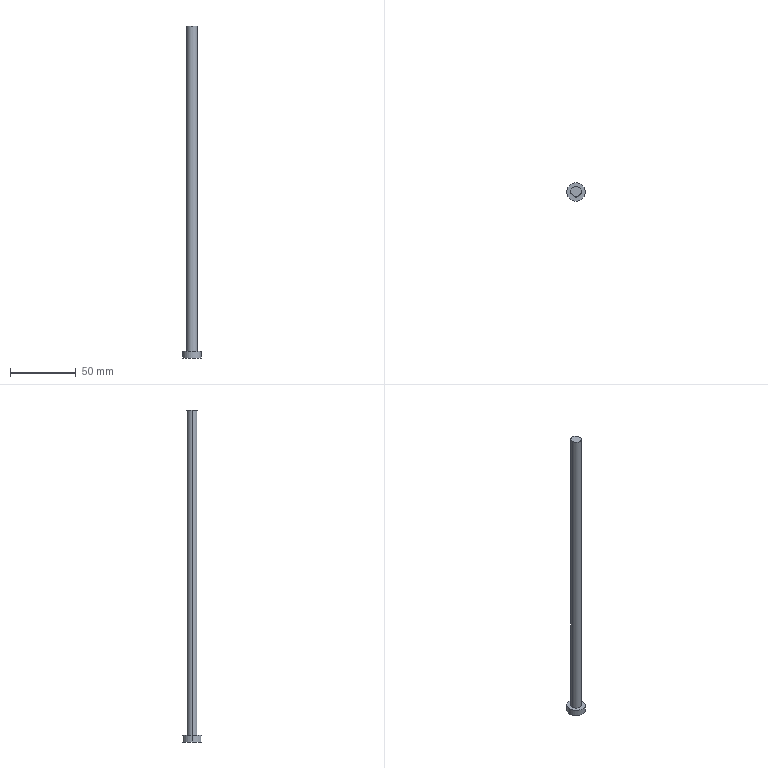Part | Creo | 1 solid | 7 faces | box 14 x 14 x 252.352 mm | volume 13203 mm3 | cylinder 4 | plane 3 | commonest cylinder face diameters 8 x2 14 x2
STEP:
#1=CARTESIAN_POINT('',(4.,0.,26.852));
#2=VERTEX_POINT('',#1);
#3=CARTESIAN_POINT('',(-4.,0.,26.852));
#4=VERTEX_POINT('',#3);
#5=CARTESIAN_POINT('',(0.,0.,26.852));
#6=DIRECTION('',(0.,0.,1.));
#7=DIRECTION('',(1.,0.,0.));
#8=AXIS2_PLACEMENT_3D('',#5,#6,#7);
#9=CIRCLE('',#8,4.);
#10=EDGE_CURVE('',#2,#4,#9,.T.);
#11=ORIENTED_EDGE('',*,*,#10,.T.);
#12=CARTESIAN_POINT('',(-4.,0.,-220.5));
#13=VERTEX_POINT('',#12);
#14=CARTESIAN_POINT('',(-4.,0.,26.852));
#15=DIRECTION('',(0.,0.,-1.));
#16=VECTOR('',#15,247.352);
#17=LINE('',#14,#16);
#18=EDGE_CURVE('',#4,#13,#17,.T.);
#19=ORIENTED_EDGE('',*,*,#18,.T.);
#20=CARTESIAN_POINT('',(4.,0.,-220.5));
#21=VERTEX_POINT('',#20);
#22=CARTESIAN_POINT('',(0.,0.,-220.5));
#23=DIRECTION('',(0.,0.,-1.));
#24=DIRECTION('',(-1.,0.,0.));
#25=AXIS2_PLACEMENT_3D('',#22,#23,#24);
#26=CIRCLE('',#25,4.);
#27=EDGE_CURVE('',#13,#21,#26,.T.);
#28=ORIENTED_EDGE('',*,*,#27,.T.);
#29=CARTESIAN_POINT('',(4.,0.,26.852));
#30=DIRECTION('',(0.,0.,-1.));
#31=VECTOR('',#30,247.352);
#32=LINE('',#29,#31);
#33=EDGE_CURVE('',#2,#21,#32,.T.);
#34=ORIENTED_EDGE('',*,*,#33,.F.);
#35=EDGE_LOOP('',(#11,#19,#28,#34));
#36=FACE_OUTER_BOUND('',#35,.F.);
#37=CARTESIAN_POINT('',(0.,0.,49.5));
#38=DIRECTION('',(0.,0.,-1.));
#39=DIRECTION('',(-1.,0.,0.));
#40=AXIS2_PLACEMENT_3D('',#37,#38,#39);
#41=CYLINDRICAL_SURFACE('',#40,4.);
#42=ADVANCED_FACE('',(#36),#41,.T.);
#43=CARTESIAN_POINT('',(0.,0.,26.852));
#44=DIRECTION('',(0.,0.,1.));
#45=DIRECTION('',(-1.,0.,0.));
#46=AXIS2_PLACEMENT_3D('',#43,#44,#45);
#47=CIRCLE('',#46,4.);
#48=EDGE_CURVE('',#4,#2,#47,.T.);
#49=ORIENTED_EDGE('',*,*,#48,.F.);
#50=ORIENTED_EDGE('',*,*,#10,.F.);
#51=EDGE_LOOP('',(#49,#50));
#52=FACE_OUTER_BOUND('',#51,.F.);
#53=CARTESIAN_POINT('',(0.,0.,26.852));
#54=DIRECTION('',(0.,0.,-1.));
#55=DIRECTION('',(-1.,0.,0.));
#56=AXIS2_PLACEMENT_3D('',#53,#54,#55);
#57=PLANE('',#56);
#58=ADVANCED_FACE('',(#52),#57,.F.);
#59=ORIENTED_EDGE('',*,*,#48,.T.);
#60=ORIENTED_EDGE('',*,*,#33,.T.);
#61=CARTESIAN_POINT('',(0.,0.,-220.5));
#62=DIRECTION('',(0.,0.,-1.));
#63=DIRECTION('',(1.,0.,0.));
#64=AXIS2_PLACEMENT_3D('',#61,#62,#63);
#65=CIRCLE('',#64,4.);
#66=EDGE_CURVE('',#21,#13,#65,.T.);
#67=ORIENTED_EDGE('',*,*,#66,.T.);
#68=ORIENTED_EDGE('',*,*,#18,.F.);
#69=EDGE_LOOP('',(#59,#60,#67,#68));
#70=FACE_OUTER_BOUND('',#69,.F.);
#71=CARTESIAN_POINT('',(0.,0.,49.5));
#72=DIRECTION('',(0.,0.,-1.));
#73=DIRECTION('',(-1.,0.,0.));
#74=AXIS2_PLACEMENT_3D('',#71,#72,#73);
#75=CYLINDRICAL_SURFACE('',#74,4.);
#76=ADVANCED_FACE('',(#70),#75,.T.);
#77=CARTESIAN_POINT('',(-7.,0.,-220.5));
#78=VERTEX_POINT('',#77);
#79=CARTESIAN_POINT('',(7.,0.,-220.5));
#80=VERTEX_POINT('',#79);
#81=CARTESIAN_POINT('',(0.,0.,-220.5));
#82=DIRECTION('',(0.,0.,1.));
#83=DIRECTION('',(-1.,0.,0.));
#84=AXIS2_PLACEMENT_3D('',#81,#82,#83);
#85=CIRCLE('',#84,7.);
#86=EDGE_CURVE('',#78,#80,#85,.T.);
#87=ORIENTED_EDGE('',*,*,#86,.F.);
#88=CARTESIAN_POINT('',(0.,0.,-220.5));
#89=DIRECTION('',(0.,0.,1.));
#90=DIRECTION('',(1.,0.,0.));
#91=AXIS2_PLACEMENT_3D('',#88,#89,#90);
#92=CIRCLE('',#91,7.);
#93=EDGE_CURVE('',#80,#78,#92,.T.);
#94=ORIENTED_EDGE('',*,*,#93,.F.);
#95=EDGE_LOOP('',(#87,#94));
#96=FACE_OUTER_BOUND('',#95,.F.);
#97=ORIENTED_EDGE('',*,*,#27,.F.);
#98=ORIENTED_EDGE('',*,*,#66,.F.);
#99=EDGE_LOOP('',(#97,#98));
#100=FACE_BOUND('',#99,.F.);
#101=CARTESIAN_POINT('',(0.,0.,-220.5));
#102=DIRECTION('',(0.,0.,-1.));
#103=DIRECTION('',(-1.,0.,0.));
#104=AXIS2_PLACEMENT_3D('',#101,#102,#103);
#105=PLANE('',#104);
#106=ADVANCED_FACE('',(#96,#100),#105,.F.);
#107=CARTESIAN_POINT('',(7.,0.,-225.5));
#108=VERTEX_POINT('',#107);
#109=CARTESIAN_POINT('',(-7.,0.,-225.5));
#110=VERTEX_POINT('',#109);
#111=CARTESIAN_POINT('',(0.,0.,-225.5));
#112=DIRECTION('',(0.,0.,-1.));
#113=DIRECTION('',(1.,0.,0.));
#114=AXIS2_PLACEMENT_3D('',#111,#112,#113);
#115=CIRCLE('',#114,7.);
#116=EDGE_CURVE('',#108,#110,#115,.T.);
#117=ORIENTED_EDGE('',*,*,#116,.T.);
#118=CARTESIAN_POINT('',(-7.,0.,-220.5));
#119=DIRECTION('',(0.,0.,-1.));
#120=VECTOR('',#119,5.);
#121=LINE('',#118,#120);
#122=EDGE_CURVE('',#78,#110,#121,.T.);
#123=ORIENTED_EDGE('',*,*,#122,.F.);
#124=ORIENTED_EDGE('',*,*,#86,.T.);
#125=CARTESIAN_POINT('',(7.,0.,-220.5));
#126=DIRECTION('',(0.,0.,-1.));
#127=VECTOR('',#126,5.);
#128=LINE('',#125,#127);
#129=EDGE_CURVE('',#80,#108,#128,.T.);
#130=ORIENTED_EDGE('',*,*,#129,.T.);
#131=EDGE_LOOP('',(#117,#123,#124,#130));
#132=FACE_OUTER_BOUND('',#131,.F.);
#133=CARTESIAN_POINT('',(0.,0.,-235.913));
#134=DIRECTION('',(0.,0.,-1.));
#135=DIRECTION('',(-1.,0.,0.));
#136=AXIS2_PLACEMENT_3D('',#133,#134,#135);
#137=CYLINDRICAL_SURFACE('',#136,7.);
#138=ADVANCED_FACE('',(#132),#137,.T.);
#139=CARTESIAN_POINT('',(0.,0.,-225.5));
#140=DIRECTION('',(0.,0.,-1.));
#141=DIRECTION('',(-1.,0.,0.));
#142=AXIS2_PLACEMENT_3D('',#139,#140,#141);
#143=CIRCLE('',#142,7.);
#144=EDGE_CURVE('',#110,#108,#143,.T.);
#145=ORIENTED_EDGE('',*,*,#144,.F.);
#146=ORIENTED_EDGE('',*,*,#116,.F.);
#147=EDGE_LOOP('',(#145,#146));
#148=FACE_OUTER_BOUND('',#147,.F.);
#149=CARTESIAN_POINT('',(4.,0.,-225.5));
#150=DIRECTION('',(0.,0.,1.));
#151=DIRECTION('',(1.,0.,0.));
#152=AXIS2_PLACEMENT_3D('',#149,#150,#151);
#153=PLANE('',#152);
#154=ADVANCED_FACE('',(#148),#153,.F.);
#155=ORIENTED_EDGE('',*,*,#144,.T.);
#156=ORIENTED_EDGE('',*,*,#129,.F.);
#157=ORIENTED_EDGE('',*,*,#93,.T.);
#158=ORIENTED_EDGE('',*,*,#122,.T.);
#159=EDGE_LOOP('',(#155,#156,#157,#158));
#160=FACE_OUTER_BOUND('',#159,.F.);
#161=CARTESIAN_POINT('',(0.,0.,-235.913));
#162=DIRECTION('',(0.,0.,-1.));
#163=DIRECTION('',(-1.,0.,0.));
#164=AXIS2_PLACEMENT_3D('',#161,#162,#163);
#165=CYLINDRICAL_SURFACE('',#164,7.);
#166=ADVANCED_FACE('',(#160),#165,.T.);
#167=CLOSED_SHELL('',(#42,#58,#76,#106,#138,#154,#166));
#168=MANIFOLD_SOLID_BREP('',#167);
#169=(LENGTH_UNIT()NAMED_UNIT(*)SI_UNIT(.MILLI.,.METRE.));
#170=UNCERTAINTY_MEASURE_WITH_UNIT(LENGTH_MEASURE(0.02531),#169,'','');
#171=(NAMED_UNIT(*)PLANE_ANGLE_UNIT()SI_UNIT($,.RADIAN.));
#172=PLANE_ANGLE_MEASURE_WITH_UNIT(PLANE_ANGLE_MEASURE(0.01745),#171);
#173=(CONVERSION_BASED_UNIT('DEGREE',#172)NAMED_UNIT(*)PLANE_ANGLE_UNIT());
#174=(NAMED_UNIT(*)SI_UNIT($,.STERADIAN.)SOLID_ANGLE_UNIT());
#175=(GEOMETRIC_REPRESENTATION_CONTEXT(3)GLOBAL_UNCERTAINTY_ASSIGNED_CONTEXT((#170))GLOBAL_UNIT_ASSIGNED_CONTEXT((#169,#173,#174))REPRESENTATION_CONTEXT('',''));
#176=ADVANCED_BREP_SHAPE_REPRESENTATION('',(#168),#175);